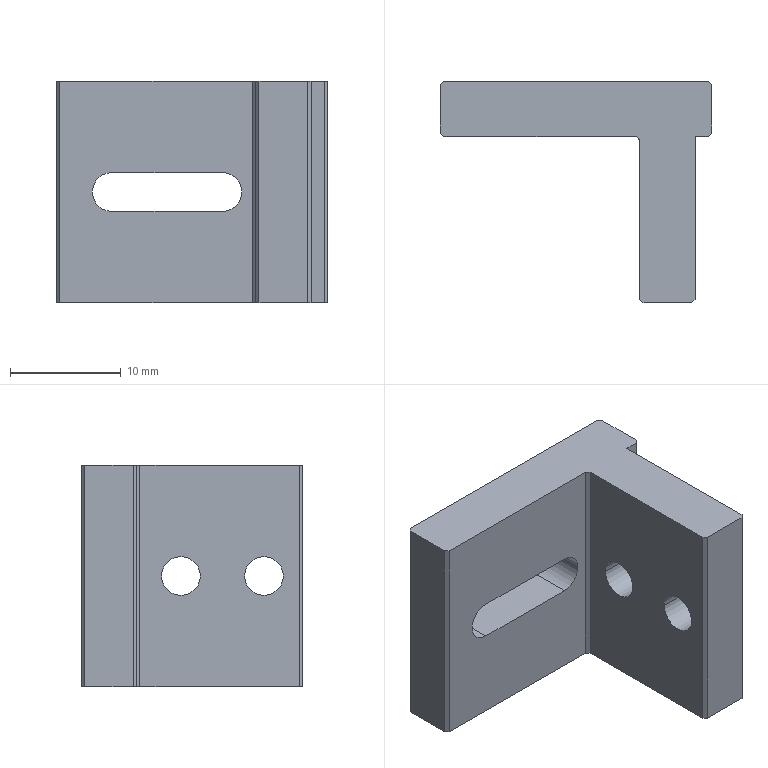Part | SolidWorks | features ICE 2, Extrusion 1 | 1 solid | 26 faces | box 24.5 x 20 x 20 mm | volume 3626 mm3 | plane 19 | cylinder 7 | commonest cylinder face diameters 3.5 x7
STEP:
#1=CARTESIAN_POINT('',(-9.5,5.,11.75));
#2=VERTEX_POINT('',#1);
#3=CARTESIAN_POINT('',(-7.75,5.,10.));
#4=VERTEX_POINT('',#3);
#5=CARTESIAN_POINT('',(-9.5,5.,10.));
#6=DIRECTION('',(0.,1.,0.));
#7=DIRECTION('',(1.,0.,0.));
#8=AXIS2_PLACEMENT_3D('',#5,#6,#7);
#9=CIRCLE('',#8,1.75);
#10=EDGE_CURVE('',#2,#4,#9,.T.);
#11=ORIENTED_EDGE('',*,*,#10,.T.);
#12=CARTESIAN_POINT('',(-7.75,0.,10.));
#13=VERTEX_POINT('',#12);
#14=CARTESIAN_POINT('',(-7.75,5.001,10.));
#15=DIRECTION('',(0.,-1.,0.));
#16=VECTOR('',#15,1000.);
#17=LINE('',#14,#16);
#18=EDGE_CURVE('',#4,#13,#17,.T.);
#19=ORIENTED_EDGE('',*,*,#18,.T.);
#20=CARTESIAN_POINT('',(-9.5,0.,11.75));
#21=VERTEX_POINT('',#20);
#22=CARTESIAN_POINT('',(-9.5,0.,10.));
#23=DIRECTION('',(0.,-1.,0.));
#24=DIRECTION('',(1.,0.,0.));
#25=AXIS2_PLACEMENT_3D('',#22,#23,#24);
#26=CIRCLE('',#25,1.75);
#27=EDGE_CURVE('',#13,#21,#26,.T.);
#28=ORIENTED_EDGE('',*,*,#27,.T.);
#29=CARTESIAN_POINT('',(-9.5,5.001,11.75));
#30=DIRECTION('',(0.,-1.,0.));
#31=VECTOR('',#30,1000.);
#32=LINE('',#29,#31);
#33=EDGE_CURVE('',#2,#21,#32,.T.);
#34=ORIENTED_EDGE('',*,*,#33,.F.);
#35=EDGE_LOOP('',(#11,#19,#28,#34));
#36=FACE_OUTER_BOUND('',#35,.T.);
#37=CARTESIAN_POINT('',(-9.5,5.001,10.));
#38=DIRECTION('',(0.,-1.,0.));
#39=DIRECTION('',(1.,0.,0.));
#40=AXIS2_PLACEMENT_3D('',#37,#38,#39);
#41=CYLINDRICAL_SURFACE('',#40,1.75);
#42=ADVANCED_FACE('',(#36),#41,.F.);
#43=CARTESIAN_POINT('',(-6.5,-9.75,10.));
#44=VERTEX_POINT('',#43);
#45=CARTESIAN_POINT('',(-6.5,-13.25,10.));
#46=VERTEX_POINT('',#45);
#47=CARTESIAN_POINT('',(-6.5,-11.5,10.));
#48=DIRECTION('',(-1.,0.,0.));
#49=DIRECTION('',(0.,1.,0.));
#50=AXIS2_PLACEMENT_3D('',#47,#48,#49);
#51=CIRCLE('',#50,1.75);
#52=EDGE_CURVE('',#44,#46,#51,.T.);
#53=ORIENTED_EDGE('',*,*,#52,.T.);
#54=CARTESIAN_POINT('',(-1.5,-13.25,10.));
#55=VERTEX_POINT('',#54);
#56=CARTESIAN_POINT('',(-24.501,-13.25,10.));
#57=DIRECTION('',(1.,0.,0.));
#58=VECTOR('',#57,1000.);
#59=LINE('',#56,#58);
#60=EDGE_CURVE('',#46,#55,#59,.T.);
#61=ORIENTED_EDGE('',*,*,#60,.T.);
#62=CARTESIAN_POINT('',(-1.5,-9.75,10.));
#63=VERTEX_POINT('',#62);
#64=CARTESIAN_POINT('',(-1.5,-11.5,10.));
#65=DIRECTION('',(1.,0.,0.));
#66=DIRECTION('',(0.,1.,0.));
#67=AXIS2_PLACEMENT_3D('',#64,#65,#66);
#68=CIRCLE('',#67,1.75);
#69=EDGE_CURVE('',#55,#63,#68,.T.);
#70=ORIENTED_EDGE('',*,*,#69,.T.);
#71=CARTESIAN_POINT('',(-24.501,-9.75,10.));
#72=DIRECTION('',(1.,0.,0.));
#73=VECTOR('',#72,1000.);
#74=LINE('',#71,#73);
#75=EDGE_CURVE('',#44,#63,#74,.T.);
#76=ORIENTED_EDGE('',*,*,#75,.F.);
#77=EDGE_LOOP('',(#53,#61,#70,#76));
#78=FACE_OUTER_BOUND('',#77,.T.);
#79=CARTESIAN_POINT('',(-24.501,-11.5,10.));
#80=DIRECTION('',(1.,0.,0.));
#81=DIRECTION('',(0.,1.,0.));
#82=AXIS2_PLACEMENT_3D('',#79,#80,#81);
#83=CYLINDRICAL_SURFACE('',#82,1.75);
#84=ADVANCED_FACE('',(#78),#83,.F.);
#85=CARTESIAN_POINT('',(-6.5,-2.25,10.));
#86=VERTEX_POINT('',#85);
#87=CARTESIAN_POINT('',(-6.5,-5.75,10.));
#88=VERTEX_POINT('',#87);
#89=CARTESIAN_POINT('',(-6.5,-4.,10.));
#90=DIRECTION('',(-1.,0.,0.));
#91=DIRECTION('',(0.,1.,0.));
#92=AXIS2_PLACEMENT_3D('',#89,#90,#91);
#93=CIRCLE('',#92,1.75);
#94=EDGE_CURVE('',#86,#88,#93,.T.);
#95=ORIENTED_EDGE('',*,*,#94,.T.);
#96=CARTESIAN_POINT('',(-1.5,-5.75,10.));
#97=VERTEX_POINT('',#96);
#98=CARTESIAN_POINT('',(-24.501,-5.75,10.));
#99=DIRECTION('',(1.,0.,0.));
#100=VECTOR('',#99,1000.);
#101=LINE('',#98,#100);
#102=EDGE_CURVE('',#88,#97,#101,.T.);
#103=ORIENTED_EDGE('',*,*,#102,.T.);
#104=CARTESIAN_POINT('',(-1.5,-2.25,10.));
#105=VERTEX_POINT('',#104);
#106=CARTESIAN_POINT('',(-1.5,-4.,10.));
#107=DIRECTION('',(1.,0.,0.));
#108=DIRECTION('',(0.,-1.,0.));
#109=AXIS2_PLACEMENT_3D('',#106,#107,#108);
#110=CIRCLE('',#109,1.75);
#111=EDGE_CURVE('',#97,#105,#110,.T.);
#112=ORIENTED_EDGE('',*,*,#111,.T.);
#113=CARTESIAN_POINT('',(-24.501,-2.25,10.));
#114=DIRECTION('',(1.,0.,0.));
#115=VECTOR('',#114,1000.);
#116=LINE('',#113,#115);
#117=EDGE_CURVE('',#86,#105,#116,.T.);
#118=ORIENTED_EDGE('',*,*,#117,.F.);
#119=EDGE_LOOP('',(#95,#103,#112,#118));
#120=FACE_OUTER_BOUND('',#119,.T.);
#121=CARTESIAN_POINT('',(-24.501,-4.,10.));
#122=DIRECTION('',(1.,0.,0.));
#123=DIRECTION('',(0.,1.,0.));
#124=AXIS2_PLACEMENT_3D('',#121,#122,#123);
#125=CYLINDRICAL_SURFACE('',#124,1.75);
#126=ADVANCED_FACE('',(#120),#125,.F.);
#127=CARTESIAN_POINT('',(-1.5,-11.5,10.));
#128=DIRECTION('',(1.,0.,0.));
#129=DIRECTION('',(0.,1.,0.));
#130=AXIS2_PLACEMENT_3D('',#127,#128,#129);
#131=CIRCLE('',#130,1.75);
#132=EDGE_CURVE('',#63,#55,#131,.T.);
#133=ORIENTED_EDGE('',*,*,#132,.F.);
#134=ORIENTED_EDGE('',*,*,#69,.F.);
#135=EDGE_LOOP('',(#133,#134));
#136=FACE_BOUND('',#135,.T.);
#137=CARTESIAN_POINT('',(-1.5,-4.,10.));
#138=DIRECTION('',(1.,0.,0.));
#139=DIRECTION('',(0.,-1.,0.));
#140=AXIS2_PLACEMENT_3D('',#137,#138,#139);
#141=CIRCLE('',#140,1.75);
#142=EDGE_CURVE('',#105,#97,#141,.T.);
#143=ORIENTED_EDGE('',*,*,#142,.F.);
#144=ORIENTED_EDGE('',*,*,#111,.F.);
#145=EDGE_LOOP('',(#143,#144));
#146=FACE_BOUND('',#145,.T.);
#147=CARTESIAN_POINT('',(-1.5,-14.7,0.));
#148=VERTEX_POINT('',#147);
#149=CARTESIAN_POINT('',(-1.5,0.,0.));
#150=VERTEX_POINT('',#149);
#151=CARTESIAN_POINT('',(-1.5,0.,0.));
#152=DIRECTION('',(0.,1.,0.));
#153=VECTOR('',#152,1000.);
#154=LINE('',#151,#153);
#155=EDGE_CURVE('',#148,#150,#154,.T.);
#156=ORIENTED_EDGE('',*,*,#155,.T.);
#157=CARTESIAN_POINT('',(-1.5,0.,20.));
#158=VERTEX_POINT('',#157);
#159=CARTESIAN_POINT('',(-1.5,0.,20.));
#160=DIRECTION('',(0.,0.,-1.));
#161=VECTOR('',#160,1000.);
#162=LINE('',#159,#161);
#163=EDGE_CURVE('',#158,#150,#162,.T.);
#164=ORIENTED_EDGE('',*,*,#163,.F.);
#165=CARTESIAN_POINT('',(-1.5,-14.7,20.));
#166=VERTEX_POINT('',#165);
#167=CARTESIAN_POINT('',(-1.5,0.,20.));
#168=DIRECTION('',(0.,1.,0.));
#169=VECTOR('',#168,1000.);
#170=LINE('',#167,#169);
#171=EDGE_CURVE('',#166,#158,#170,.T.);
#172=ORIENTED_EDGE('',*,*,#171,.F.);
#173=CARTESIAN_POINT('',(-1.5,-14.7,20.));
#174=DIRECTION('',(0.,0.,-1.));
#175=VECTOR('',#174,1000.);
#176=LINE('',#173,#175);
#177=EDGE_CURVE('',#166,#148,#176,.T.);
#178=ORIENTED_EDGE('',*,*,#177,.T.);
#179=EDGE_LOOP('',(#156,#164,#172,#178));
#180=FACE_OUTER_BOUND('',#179,.T.);
#181=CARTESIAN_POINT('',(-1.5,0.,20.));
#182=DIRECTION('',(-1.,0.,0.));
#183=DIRECTION('',(0.,-1.,0.));
#184=AXIS2_PLACEMENT_3D('',#181,#182,#183);
#185=PLANE('',#184);
#186=ADVANCED_FACE('',(#136,#146,#180),#185,.F.);
#187=CARTESIAN_POINT('',(-0.3,0.,0.));
#188=VERTEX_POINT('',#187);
#189=CARTESIAN_POINT('',(-0.3,0.,0.));
#190=DIRECTION('',(1.,0.,0.));
#191=VECTOR('',#190,1000.);
#192=LINE('',#189,#191);
#193=EDGE_CURVE('',#150,#188,#192,.T.);
#194=ORIENTED_EDGE('',*,*,#193,.T.);
#195=CARTESIAN_POINT('',(-0.3,0.,20.));
#196=VERTEX_POINT('',#195);
#197=CARTESIAN_POINT('',(-0.3,0.,20.));
#198=DIRECTION('',(0.,0.,-1.));
#199=VECTOR('',#198,1000.);
#200=LINE('',#197,#199);
#201=EDGE_CURVE('',#196,#188,#200,.T.);
#202=ORIENTED_EDGE('',*,*,#201,.F.);
#203=CARTESIAN_POINT('',(-0.3,0.,20.));
#204=DIRECTION('',(1.,0.,0.));
#205=VECTOR('',#204,1000.);
#206=LINE('',#203,#205);
#207=EDGE_CURVE('',#158,#196,#206,.T.);
#208=ORIENTED_EDGE('',*,*,#207,.F.);
#209=ORIENTED_EDGE('',*,*,#163,.T.);
#210=EDGE_LOOP('',(#194,#202,#208,#209));
#211=FACE_OUTER_BOUND('',#210,.T.);
#212=CARTESIAN_POINT('',(-0.3,0.,20.));
#213=DIRECTION('',(0.,1.,0.));
#214=DIRECTION('',(-1.,0.,0.));
#215=AXIS2_PLACEMENT_3D('',#212,#213,#214);
#216=PLANE('',#215);
#217=ADVANCED_FACE('',(#211),#216,.F.);
#218=CARTESIAN_POINT('',(0.,0.3,0.));
#219=VERTEX_POINT('',#218);
#220=CARTESIAN_POINT('',(0.,0.3,0.));
#221=DIRECTION('',(0.7071,0.7071,0.));
#222=VECTOR('',#221,1000.);
#223=LINE('',#220,#222);
#224=EDGE_CURVE('',#188,#219,#223,.T.);
#225=ORIENTED_EDGE('',*,*,#224,.T.);
#226=CARTESIAN_POINT('',(0.,0.3,20.));
#227=VERTEX_POINT('',#226);
#228=CARTESIAN_POINT('',(0.,0.3,20.));
#229=DIRECTION('',(0.,0.,-1.));
#230=VECTOR('',#229,1000.);
#231=LINE('',#228,#230);
#232=EDGE_CURVE('',#227,#219,#231,.T.);
#233=ORIENTED_EDGE('',*,*,#232,.F.);
#234=CARTESIAN_POINT('',(0.,0.3,20.));
#235=DIRECTION('',(0.7071,0.7071,0.));
#236=VECTOR('',#235,1000.);
#237=LINE('',#234,#236);
#238=EDGE_CURVE('',#196,#227,#237,.T.);
#239=ORIENTED_EDGE('',*,*,#238,.F.);
#240=ORIENTED_EDGE('',*,*,#201,.T.);
#241=EDGE_LOOP('',(#225,#233,#239,#240));
#242=FACE_OUTER_BOUND('',#241,.T.);
#243=CARTESIAN_POINT('',(0.,0.3,20.));
#244=DIRECTION('',(-0.7071,0.7071,0.));
#245=DIRECTION('',(-0.7071,-0.7071,0.));
#246=AXIS2_PLACEMENT_3D('',#243,#244,#245);
#247=PLANE('',#246);
#248=ADVANCED_FACE('',(#242),#247,.F.);
#249=CARTESIAN_POINT('',(0.,4.7,0.));
#250=VERTEX_POINT('',#249);
#251=CARTESIAN_POINT('',(0.,0.3,0.));
#252=DIRECTION('',(0.,1.,0.));
#253=VECTOR('',#252,1000.);
#254=LINE('',#251,#253);
#255=EDGE_CURVE('',#219,#250,#254,.T.);
#256=ORIENTED_EDGE('',*,*,#255,.T.);
#257=CARTESIAN_POINT('',(0.,4.7,20.));
#258=VERTEX_POINT('',#257);
#259=CARTESIAN_POINT('',(0.,4.7,20.));
#260=DIRECTION('',(0.,0.,-1.));
#261=VECTOR('',#260,1000.);
#262=LINE('',#259,#261);
#263=EDGE_CURVE('',#258,#250,#262,.T.);
#264=ORIENTED_EDGE('',*,*,#263,.F.);
#265=CARTESIAN_POINT('',(0.,0.3,20.));
#266=DIRECTION('',(0.,1.,0.));
#267=VECTOR('',#266,1000.);
#268=LINE('',#265,#267);
#269=EDGE_CURVE('',#227,#258,#268,.T.);
#270=ORIENTED_EDGE('',*,*,#269,.F.);
#271=ORIENTED_EDGE('',*,*,#232,.T.);
#272=EDGE_LOOP('',(#256,#264,#270,#271));
#273=FACE_OUTER_BOUND('',#272,.T.);
#274=CARTESIAN_POINT('',(0.,0.3,20.));
#275=DIRECTION('',(-1.,0.,0.));
#276=DIRECTION('',(0.,0.,1.));
#277=AXIS2_PLACEMENT_3D('',#274,#275,#276);
#278=PLANE('',#277);
#279=ADVANCED_FACE('',(#273),#278,.F.);
#280=CARTESIAN_POINT('',(-0.3,5.,0.));
#281=VERTEX_POINT('',#280);
#282=CARTESIAN_POINT('',(0.,4.7,0.));
#283=DIRECTION('',(-0.7071,0.7071,0.));
#284=VECTOR('',#283,1000.);
#285=LINE('',#282,#284);
#286=EDGE_CURVE('',#250,#281,#285,.T.);
#287=ORIENTED_EDGE('',*,*,#286,.T.);
#288=CARTESIAN_POINT('',(-0.3,5.,20.));
#289=VERTEX_POINT('',#288);
#290=CARTESIAN_POINT('',(-0.3,5.,20.));
#291=DIRECTION('',(0.,0.,-1.));
#292=VECTOR('',#291,1000.);
#293=LINE('',#290,#292);
#294=EDGE_CURVE('',#289,#281,#293,.T.);
#295=ORIENTED_EDGE('',*,*,#294,.F.);
#296=CARTESIAN_POINT('',(0.,4.7,20.));
#297=DIRECTION('',(-0.7071,0.7071,0.));
#298=VECTOR('',#297,1000.);
#299=LINE('',#296,#298);
#300=EDGE_CURVE('',#258,#289,#299,.T.);
#301=ORIENTED_EDGE('',*,*,#300,.F.);
#302=ORIENTED_EDGE('',*,*,#263,.T.);
#303=EDGE_LOOP('',(#287,#295,#301,#302));
#304=FACE_OUTER_BOUND('',#303,.T.);
#305=CARTESIAN_POINT('',(0.,4.7,20.));
#306=DIRECTION('',(-0.7071,-0.7071,0.));
#307=DIRECTION('',(0.7071,-0.7071,0.));
#308=AXIS2_PLACEMENT_3D('',#305,#306,#307);
#309=PLANE('',#308);
#310=ADVANCED_FACE('',(#304),#309,.F.);
#311=CARTESIAN_POINT('',(-19.5,5.,11.75));
#312=VERTEX_POINT('',#311);
#313=CARTESIAN_POINT('',(-19.5,5.,11.75));
#314=DIRECTION('',(1.,0.,0.));
#315=VECTOR('',#314,1000.);
#316=LINE('',#313,#315);
#317=EDGE_CURVE('',#312,#2,#316,.T.);
#318=ORIENTED_EDGE('',*,*,#317,.F.);
#319=CARTESIAN_POINT('',(-19.5,5.,8.25));
#320=VERTEX_POINT('',#319);
#321=CARTESIAN_POINT('',(-19.5,5.,10.));
#322=DIRECTION('',(0.,1.,0.));
#323=DIRECTION('',(1.,0.,0.));
#324=AXIS2_PLACEMENT_3D('',#321,#322,#323);
#325=CIRCLE('',#324,1.75);
#326=EDGE_CURVE('',#320,#312,#325,.T.);
#327=ORIENTED_EDGE('',*,*,#326,.F.);
#328=CARTESIAN_POINT('',(-9.5,5.,8.25));
#329=VERTEX_POINT('',#328);
#330=CARTESIAN_POINT('',(-19.5,5.,8.25));
#331=DIRECTION('',(-1.,0.,0.));
#332=VECTOR('',#331,1000.);
#333=LINE('',#330,#332);
#334=EDGE_CURVE('',#329,#320,#333,.T.);
#335=ORIENTED_EDGE('',*,*,#334,.F.);
#336=CARTESIAN_POINT('',(-9.5,5.,10.));
#337=DIRECTION('',(0.,1.,0.));
#338=DIRECTION('',(1.,0.,0.));
#339=AXIS2_PLACEMENT_3D('',#336,#337,#338);
#340=CIRCLE('',#339,1.75);
#341=EDGE_CURVE('',#4,#329,#340,.T.);
#342=ORIENTED_EDGE('',*,*,#341,.F.);
#343=ORIENTED_EDGE('',*,*,#10,.F.);
#344=EDGE_LOOP('',(#318,#327,#335,#342,#343));
#345=FACE_BOUND('',#344,.T.);
#346=CARTESIAN_POINT('',(-24.2,5.,0.));
#347=VERTEX_POINT('',#346);
#348=CARTESIAN_POINT('',(-0.3,5.,0.));
#349=DIRECTION('',(-1.,0.,0.));
#350=VECTOR('',#349,1000.);
#351=LINE('',#348,#350);
#352=EDGE_CURVE('',#281,#347,#351,.T.);
#353=ORIENTED_EDGE('',*,*,#352,.T.);
#354=CARTESIAN_POINT('',(-24.2,5.,20.));
#355=VERTEX_POINT('',#354);
#356=CARTESIAN_POINT('',(-24.2,5.,20.));
#357=DIRECTION('',(0.,0.,-1.));
#358=VECTOR('',#357,1000.);
#359=LINE('',#356,#358);
#360=EDGE_CURVE('',#355,#347,#359,.T.);
#361=ORIENTED_EDGE('',*,*,#360,.F.);
#362=CARTESIAN_POINT('',(-0.3,5.,20.));
#363=DIRECTION('',(-1.,0.,0.));
#364=VECTOR('',#363,1000.);
#365=LINE('',#362,#364);
#366=EDGE_CURVE('',#289,#355,#365,.T.);
#367=ORIENTED_EDGE('',*,*,#366,.F.);
#368=ORIENTED_EDGE('',*,*,#294,.T.);
#369=EDGE_LOOP('',(#353,#361,#367,#368));
#370=FACE_OUTER_BOUND('',#369,.T.);
#371=CARTESIAN_POINT('',(-0.3,5.,20.));
#372=DIRECTION('',(0.,-1.,0.));
#373=DIRECTION('',(1.,0.,0.));
#374=AXIS2_PLACEMENT_3D('',#371,#372,#373);
#375=PLANE('',#374);
#376=ADVANCED_FACE('',(#345,#370),#375,.F.);
#377=CARTESIAN_POINT('',(-24.5,4.7,0.));
#378=VERTEX_POINT('',#377);
#379=CARTESIAN_POINT('',(-24.2,5.,0.));
#380=DIRECTION('',(-0.7071,-0.7071,0.));
#381=VECTOR('',#380,1000.);
#382=LINE('',#379,#381);
#383=EDGE_CURVE('',#347,#378,#382,.T.);
#384=ORIENTED_EDGE('',*,*,#383,.T.);
#385=CARTESIAN_POINT('',(-24.5,4.7,20.));
#386=VERTEX_POINT('',#385);
#387=CARTESIAN_POINT('',(-24.5,4.7,20.));
#388=DIRECTION('',(0.,0.,-1.));
#389=VECTOR('',#388,1000.);
#390=LINE('',#387,#389);
#391=EDGE_CURVE('',#386,#378,#390,.T.);
#392=ORIENTED_EDGE('',*,*,#391,.F.);
#393=CARTESIAN_POINT('',(-24.2,5.,20.));
#394=DIRECTION('',(-0.7071,-0.7071,0.));
#395=VECTOR('',#394,1000.);
#396=LINE('',#393,#395);
#397=EDGE_CURVE('',#355,#386,#396,.T.);
#398=ORIENTED_EDGE('',*,*,#397,.F.);
#399=ORIENTED_EDGE('',*,*,#360,.T.);
#400=EDGE_LOOP('',(#384,#392,#398,#399));
#401=FACE_OUTER_BOUND('',#400,.T.);
#402=CARTESIAN_POINT('',(-24.2,5.,20.));
#403=DIRECTION('',(0.7071,-0.7071,0.));
#404=DIRECTION('',(0.7071,0.7071,0.));
#405=AXIS2_PLACEMENT_3D('',#402,#403,#404);
#406=PLANE('',#405);
#407=ADVANCED_FACE('',(#401),#406,.F.);
#408=CARTESIAN_POINT('',(-24.5,0.3,0.));
#409=VERTEX_POINT('',#408);
#410=CARTESIAN_POINT('',(-24.5,0.3,0.));
#411=DIRECTION('',(0.,-1.,0.));
#412=VECTOR('',#411,1000.);
#413=LINE('',#410,#412);
#414=EDGE_CURVE('',#378,#409,#413,.T.);
#415=ORIENTED_EDGE('',*,*,#414,.T.);
#416=CARTESIAN_POINT('',(-24.5,0.3,20.));
#417=VERTEX_POINT('',#416);
#418=CARTESIAN_POINT('',(-24.5,0.3,20.));
#419=DIRECTION('',(0.,0.,-1.));
#420=VECTOR('',#419,1000.);
#421=LINE('',#418,#420);
#422=EDGE_CURVE('',#417,#409,#421,.T.);
#423=ORIENTED_EDGE('',*,*,#422,.F.);
#424=CARTESIAN_POINT('',(-24.5,0.3,20.));
#425=DIRECTION('',(0.,-1.,0.));
#426=VECTOR('',#425,1000.);
#427=LINE('',#424,#426);
#428=EDGE_CURVE('',#386,#417,#427,.T.);
#429=ORIENTED_EDGE('',*,*,#428,.F.);
#430=ORIENTED_EDGE('',*,*,#391,.T.);
#431=EDGE_LOOP('',(#415,#423,#429,#430));
#432=FACE_OUTER_BOUND('',#431,.T.);
#433=CARTESIAN_POINT('',(-24.5,0.3,20.));
#434=DIRECTION('',(1.,0.,0.));
#435=DIRECTION('',(0.,0.,-1.));
#436=AXIS2_PLACEMENT_3D('',#433,#434,#435);
#437=PLANE('',#436);
#438=ADVANCED_FACE('',(#432),#437,.F.);
#439=CARTESIAN_POINT('',(-24.2,0.,0.));
#440=VERTEX_POINT('',#439);
#441=CARTESIAN_POINT('',(-24.2,0.,0.));
#442=DIRECTION('',(0.7071,-0.7071,0.));
#443=VECTOR('',#442,1000.);
#444=LINE('',#441,#443);
#445=EDGE_CURVE('',#409,#440,#444,.T.);
#446=ORIENTED_EDGE('',*,*,#445,.T.);
#447=CARTESIAN_POINT('',(-24.2,0.,20.));
#448=VERTEX_POINT('',#447);
#449=CARTESIAN_POINT('',(-24.2,0.,20.));
#450=DIRECTION('',(0.,0.,-1.));
#451=VECTOR('',#450,1000.);
#452=LINE('',#449,#451);
#453=EDGE_CURVE('',#448,#440,#452,.T.);
#454=ORIENTED_EDGE('',*,*,#453,.F.);
#455=CARTESIAN_POINT('',(-24.2,0.,20.));
#456=DIRECTION('',(0.7071,-0.7071,0.));
#457=VECTOR('',#456,1000.);
#458=LINE('',#455,#457);
#459=EDGE_CURVE('',#417,#448,#458,.T.);
#460=ORIENTED_EDGE('',*,*,#459,.F.);
#461=ORIENTED_EDGE('',*,*,#422,.T.);
#462=EDGE_LOOP('',(#446,#454,#460,#461));
#463=FACE_OUTER_BOUND('',#462,.T.);
#464=CARTESIAN_POINT('',(-24.2,0.,20.));
#465=DIRECTION('',(0.7071,0.7071,0.));
#466=DIRECTION('',(-0.7071,0.7071,0.));
#467=AXIS2_PLACEMENT_3D('',#464,#465,#466);
#468=PLANE('',#467);
#469=ADVANCED_FACE('',(#463),#468,.F.);
#470=CARTESIAN_POINT('',(-19.5,0.,8.25));
#471=VERTEX_POINT('',#470);
#472=CARTESIAN_POINT('',(-9.5,0.,8.25));
#473=VERTEX_POINT('',#472);
#474=CARTESIAN_POINT('',(-19.5,0.,8.25));
#475=DIRECTION('',(1.,0.,0.));
#476=VECTOR('',#475,1000.);
#477=LINE('',#474,#476);
#478=EDGE_CURVE('',#471,#473,#477,.T.);
#479=ORIENTED_EDGE('',*,*,#478,.F.);
#480=CARTESIAN_POINT('',(-19.5,0.,11.75));
#481=VERTEX_POINT('',#480);
#482=CARTESIAN_POINT('',(-19.5,0.,10.));
#483=DIRECTION('',(0.,-1.,0.));
#484=DIRECTION('',(1.,0.,0.));
#485=AXIS2_PLACEMENT_3D('',#482,#483,#484);
#486=CIRCLE('',#485,1.75);
#487=EDGE_CURVE('',#481,#471,#486,.T.);
#488=ORIENTED_EDGE('',*,*,#487,.F.);
#489=CARTESIAN_POINT('',(-19.5,0.,11.75));
#490=DIRECTION('',(-1.,0.,0.));
#491=VECTOR('',#490,1000.);
#492=LINE('',#489,#491);
#493=EDGE_CURVE('',#21,#481,#492,.T.);
#494=ORIENTED_EDGE('',*,*,#493,.F.);
#495=ORIENTED_EDGE('',*,*,#27,.F.);
#496=CARTESIAN_POINT('',(-9.5,0.,10.));
#497=DIRECTION('',(0.,-1.,0.));
#498=DIRECTION('',(1.,0.,0.));
#499=AXIS2_PLACEMENT_3D('',#496,#497,#498);
#500=CIRCLE('',#499,1.75);
#501=EDGE_CURVE('',#473,#13,#500,.T.);
#502=ORIENTED_EDGE('',*,*,#501,.F.);
#503=EDGE_LOOP('',(#479,#488,#494,#495,#502));
#504=FACE_BOUND('',#503,.T.);
#505=CARTESIAN_POINT('',(-6.8,0.,0.));
#506=VERTEX_POINT('',#505);
#507=CARTESIAN_POINT('',(-6.8,0.,0.));
#508=DIRECTION('',(1.,0.,0.));
#509=VECTOR('',#508,1000.);
#510=LINE('',#507,#509);
#511=EDGE_CURVE('',#440,#506,#510,.T.);
#512=ORIENTED_EDGE('',*,*,#511,.T.);
#513=CARTESIAN_POINT('',(-6.8,0.,20.));
#514=VERTEX_POINT('',#513);
#515=CARTESIAN_POINT('',(-6.8,0.,20.));
#516=DIRECTION('',(0.,0.,-1.));
#517=VECTOR('',#516,1000.);
#518=LINE('',#515,#517);
#519=EDGE_CURVE('',#514,#506,#518,.T.);
#520=ORIENTED_EDGE('',*,*,#519,.F.);
#521=CARTESIAN_POINT('',(-6.8,0.,20.));
#522=DIRECTION('',(1.,0.,0.));
#523=VECTOR('',#522,1000.);
#524=LINE('',#521,#523);
#525=EDGE_CURVE('',#448,#514,#524,.T.);
#526=ORIENTED_EDGE('',*,*,#525,.F.);
#527=ORIENTED_EDGE('',*,*,#453,.T.);
#528=EDGE_LOOP('',(#512,#520,#526,#527));
#529=FACE_OUTER_BOUND('',#528,.T.);
#530=CARTESIAN_POINT('',(-6.8,0.,20.));
#531=DIRECTION('',(0.,1.,0.));
#532=DIRECTION('',(-1.,0.,0.));
#533=AXIS2_PLACEMENT_3D('',#530,#531,#532);
#534=PLANE('',#533);
#535=ADVANCED_FACE('',(#504,#529),#534,.F.);
#536=CARTESIAN_POINT('',(-6.5,-0.3,0.));
#537=VERTEX_POINT('',#536);
#538=CARTESIAN_POINT('',(-6.5,-0.3,0.));
#539=DIRECTION('',(0.7071,-0.7071,0.));
#540=VECTOR('',#539,1000.);
#541=LINE('',#538,#540);
#542=EDGE_CURVE('',#506,#537,#541,.T.);
#543=ORIENTED_EDGE('',*,*,#542,.T.);
#544=CARTESIAN_POINT('',(-6.5,-0.3,20.));
#545=VERTEX_POINT('',#544);
#546=CARTESIAN_POINT('',(-6.5,-0.3,20.));
#547=DIRECTION('',(0.,0.,-1.));
#548=VECTOR('',#547,1000.);
#549=LINE('',#546,#548);
#550=EDGE_CURVE('',#545,#537,#549,.T.);
#551=ORIENTED_EDGE('',*,*,#550,.F.);
#552=CARTESIAN_POINT('',(-6.5,-0.3,20.));
#553=DIRECTION('',(0.7071,-0.7071,0.));
#554=VECTOR('',#553,1000.);
#555=LINE('',#552,#554);
#556=EDGE_CURVE('',#514,#545,#555,.T.);
#557=ORIENTED_EDGE('',*,*,#556,.F.);
#558=ORIENTED_EDGE('',*,*,#519,.T.);
#559=EDGE_LOOP('',(#543,#551,#557,#558));
#560=FACE_OUTER_BOUND('',#559,.T.);
#561=CARTESIAN_POINT('',(-6.5,-0.3,20.));
#562=DIRECTION('',(0.7071,0.7071,0.));
#563=DIRECTION('',(-0.7071,0.7071,0.));
#564=AXIS2_PLACEMENT_3D('',#561,#562,#563);
#565=PLANE('',#564);
#566=ADVANCED_FACE('',(#560),#565,.F.);
#567=ORIENTED_EDGE('',*,*,#52,.F.);
#568=CARTESIAN_POINT('',(-6.5,-11.5,10.));
#569=DIRECTION('',(-1.,0.,0.));
#570=DIRECTION('',(0.,1.,0.));
#571=AXIS2_PLACEMENT_3D('',#568,#569,#570);
#572=CIRCLE('',#571,1.75);
#573=EDGE_CURVE('',#46,#44,#572,.T.);
#574=ORIENTED_EDGE('',*,*,#573,.F.);
#575=EDGE_LOOP('',(#567,#574));
#576=FACE_BOUND('',#575,.T.);
#577=ORIENTED_EDGE('',*,*,#94,.F.);
#578=CARTESIAN_POINT('',(-6.5,-4.,10.));
#579=DIRECTION('',(-1.,0.,0.));
#580=DIRECTION('',(0.,1.,0.));
#581=AXIS2_PLACEMENT_3D('',#578,#579,#580);
#582=CIRCLE('',#581,1.75);
#583=EDGE_CURVE('',#88,#86,#582,.T.);
#584=ORIENTED_EDGE('',*,*,#583,.F.);
#585=EDGE_LOOP('',(#577,#584));
#586=FACE_BOUND('',#585,.T.);
#587=CARTESIAN_POINT('',(-6.5,-14.7,0.));
#588=VERTEX_POINT('',#587);
#589=CARTESIAN_POINT('',(-6.5,-0.3,0.));
#590=DIRECTION('',(0.,-1.,0.));
#591=VECTOR('',#590,1000.);
#592=LINE('',#589,#591);
#593=EDGE_CURVE('',#537,#588,#592,.T.);
#594=ORIENTED_EDGE('',*,*,#593,.T.);
#595=CARTESIAN_POINT('',(-6.5,-14.7,20.));
#596=VERTEX_POINT('',#595);
#597=CARTESIAN_POINT('',(-6.5,-14.7,20.));
#598=DIRECTION('',(0.,0.,-1.));
#599=VECTOR('',#598,1000.);
#600=LINE('',#597,#599);
#601=EDGE_CURVE('',#596,#588,#600,.T.);
#602=ORIENTED_EDGE('',*,*,#601,.F.);
#603=CARTESIAN_POINT('',(-6.5,-0.3,20.));
#604=DIRECTION('',(0.,-1.,0.));
#605=VECTOR('',#604,1000.);
#606=LINE('',#603,#605);
#607=EDGE_CURVE('',#545,#596,#606,.T.);
#608=ORIENTED_EDGE('',*,*,#607,.F.);
#609=ORIENTED_EDGE('',*,*,#550,.T.);
#610=EDGE_LOOP('',(#594,#602,#608,#609));
#611=FACE_OUTER_BOUND('',#610,.T.);
#612=CARTESIAN_POINT('',(-6.5,-0.3,20.));
#613=DIRECTION('',(1.,0.,0.));
#614=DIRECTION('',(0.,1.,0.));
#615=AXIS2_PLACEMENT_3D('',#612,#613,#614);
#616=PLANE('',#615);
#617=ADVANCED_FACE('',(#576,#586,#611),#616,.F.);
#618=CARTESIAN_POINT('',(-6.2,-15.,0.));
#619=VERTEX_POINT('',#618);
#620=CARTESIAN_POINT('',(-6.5,-14.7,0.));
#621=DIRECTION('',(0.7071,-0.7071,0.));
#622=VECTOR('',#621,1000.);
#623=LINE('',#620,#622);
#624=EDGE_CURVE('',#588,#619,#623,.T.);
#625=ORIENTED_EDGE('',*,*,#624,.T.);
#626=CARTESIAN_POINT('',(-6.2,-15.,20.));
#627=VERTEX_POINT('',#626);
#628=CARTESIAN_POINT('',(-6.2,-15.,20.));
#629=DIRECTION('',(0.,0.,-1.));
#630=VECTOR('',#629,1000.);
#631=LINE('',#628,#630);
#632=EDGE_CURVE('',#627,#619,#631,.T.);
#633=ORIENTED_EDGE('',*,*,#632,.F.);
#634=CARTESIAN_POINT('',(-6.5,-14.7,20.));
#635=DIRECTION('',(0.7071,-0.7071,0.));
#636=VECTOR('',#635,1000.);
#637=LINE('',#634,#636);
#638=EDGE_CURVE('',#596,#627,#637,.T.);
#639=ORIENTED_EDGE('',*,*,#638,.F.);
#640=ORIENTED_EDGE('',*,*,#601,.T.);
#641=EDGE_LOOP('',(#625,#633,#639,#640));
#642=FACE_OUTER_BOUND('',#641,.T.);
#643=CARTESIAN_POINT('',(-6.5,-14.7,20.));
#644=DIRECTION('',(0.7071,0.7071,0.));
#645=DIRECTION('',(-0.7071,0.7071,0.));
#646=AXIS2_PLACEMENT_3D('',#643,#644,#645);
#647=PLANE('',#646);
#648=ADVANCED_FACE('',(#642),#647,.F.);
#649=CARTESIAN_POINT('',(-1.8,-15.,0.));
#650=VERTEX_POINT('',#649);
#651=CARTESIAN_POINT('',(-6.2,-15.,0.));
#652=DIRECTION('',(1.,0.,0.));
#653=VECTOR('',#652,1000.);
#654=LINE('',#651,#653);
#655=EDGE_CURVE('',#619,#650,#654,.T.);
#656=ORIENTED_EDGE('',*,*,#655,.T.);
#657=CARTESIAN_POINT('',(-1.8,-15.,20.));
#658=VERTEX_POINT('',#657);
#659=CARTESIAN_POINT('',(-1.8,-15.,20.));
#660=DIRECTION('',(0.,0.,-1.));
#661=VECTOR('',#660,1000.);
#662=LINE('',#659,#661);
#663=EDGE_CURVE('',#658,#650,#662,.T.);
#664=ORIENTED_EDGE('',*,*,#663,.F.);
#665=CARTESIAN_POINT('',(-6.2,-15.,20.));
#666=DIRECTION('',(1.,0.,0.));
#667=VECTOR('',#666,1000.);
#668=LINE('',#665,#667);
#669=EDGE_CURVE('',#627,#658,#668,.T.);
#670=ORIENTED_EDGE('',*,*,#669,.F.);
#671=ORIENTED_EDGE('',*,*,#632,.T.);
#672=EDGE_LOOP('',(#656,#664,#670,#671));
#673=FACE_OUTER_BOUND('',#672,.T.);
#674=CARTESIAN_POINT('',(-6.2,-15.,20.));
#675=DIRECTION('',(0.,1.,0.));
#676=DIRECTION('',(0.,0.,1.));
#677=AXIS2_PLACEMENT_3D('',#674,#675,#676);
#678=PLANE('',#677);
#679=ADVANCED_FACE('',(#673),#678,.F.);
#680=CARTESIAN_POINT('',(-1.8,-15.,0.));
#681=DIRECTION('',(0.7071,0.7071,0.));
#682=VECTOR('',#681,1000.);
#683=LINE('',#680,#682);
#684=EDGE_CURVE('',#650,#148,#683,.T.);
#685=ORIENTED_EDGE('',*,*,#684,.T.);
#686=ORIENTED_EDGE('',*,*,#177,.F.);
#687=CARTESIAN_POINT('',(-1.8,-15.,20.));
#688=DIRECTION('',(0.7071,0.7071,0.));
#689=VECTOR('',#688,1000.);
#690=LINE('',#687,#689);
#691=EDGE_CURVE('',#658,#166,#690,.T.);
#692=ORIENTED_EDGE('',*,*,#691,.F.);
#693=ORIENTED_EDGE('',*,*,#663,.T.);
#694=EDGE_LOOP('',(#685,#686,#692,#693));
#695=FACE_OUTER_BOUND('',#694,.T.);
#696=CARTESIAN_POINT('',(-1.8,-15.,20.));
#697=DIRECTION('',(-0.7071,0.7071,0.));
#698=DIRECTION('',(-0.7071,-0.7071,0.));
#699=AXIS2_PLACEMENT_3D('',#696,#697,#698);
#700=PLANE('',#699);
#701=ADVANCED_FACE('',(#695),#700,.F.);
#702=ORIENTED_EDGE('',*,*,#171,.T.);
#703=ORIENTED_EDGE('',*,*,#207,.T.);
#704=ORIENTED_EDGE('',*,*,#238,.T.);
#705=ORIENTED_EDGE('',*,*,#269,.T.);
#706=ORIENTED_EDGE('',*,*,#300,.T.);
#707=ORIENTED_EDGE('',*,*,#366,.T.);
#708=ORIENTED_EDGE('',*,*,#397,.T.);
#709=ORIENTED_EDGE('',*,*,#428,.T.);
#710=ORIENTED_EDGE('',*,*,#459,.T.);
#711=ORIENTED_EDGE('',*,*,#525,.T.);
#712=ORIENTED_EDGE('',*,*,#556,.T.);
#713=ORIENTED_EDGE('',*,*,#607,.T.);
#714=ORIENTED_EDGE('',*,*,#638,.T.);
#715=ORIENTED_EDGE('',*,*,#669,.T.);
#716=ORIENTED_EDGE('',*,*,#691,.T.);
#717=EDGE_LOOP('',(#702,#703,#704,#705,#706,#707,#708,#709,#710,#711,#712,#713,#714,#715,#716));
#718=FACE_OUTER_BOUND('',#717,.T.);
#719=CARTESIAN_POINT('',(0.,0.,20.));
#720=DIRECTION('',(0.,0.,1.));
#721=DIRECTION('',(1.,0.,0.));
#722=AXIS2_PLACEMENT_3D('',#719,#720,#721);
#723=PLANE('',#722);
#724=ADVANCED_FACE('',(#718),#723,.T.);
#725=ORIENTED_EDGE('',*,*,#155,.F.);
#726=ORIENTED_EDGE('',*,*,#684,.F.);
#727=ORIENTED_EDGE('',*,*,#655,.F.);
#728=ORIENTED_EDGE('',*,*,#624,.F.);
#729=ORIENTED_EDGE('',*,*,#593,.F.);
#730=ORIENTED_EDGE('',*,*,#542,.F.);
#731=ORIENTED_EDGE('',*,*,#511,.F.);
#732=ORIENTED_EDGE('',*,*,#445,.F.);
#733=ORIENTED_EDGE('',*,*,#414,.F.);
#734=ORIENTED_EDGE('',*,*,#383,.F.);
#735=ORIENTED_EDGE('',*,*,#352,.F.);
#736=ORIENTED_EDGE('',*,*,#286,.F.);
#737=ORIENTED_EDGE('',*,*,#255,.F.);
#738=ORIENTED_EDGE('',*,*,#224,.F.);
#739=ORIENTED_EDGE('',*,*,#193,.F.);
#740=EDGE_LOOP('',(#725,#726,#727,#728,#729,#730,#731,#732,#733,#734,#735,#736,#737,#738,#739));
#741=FACE_OUTER_BOUND('',#740,.T.);
#742=CARTESIAN_POINT('',(0.,0.,0.));
#743=DIRECTION('',(0.,0.,1.));
#744=DIRECTION('',(1.,0.,0.));
#745=AXIS2_PLACEMENT_3D('',#742,#743,#744);
#746=PLANE('',#745);
#747=ADVANCED_FACE('',(#741),#746,.F.);
#748=ORIENTED_EDGE('',*,*,#102,.F.);
#749=ORIENTED_EDGE('',*,*,#583,.T.);
#750=ORIENTED_EDGE('',*,*,#117,.T.);
#751=ORIENTED_EDGE('',*,*,#142,.T.);
#752=EDGE_LOOP('',(#748,#749,#750,#751));
#753=FACE_OUTER_BOUND('',#752,.T.);
#754=CARTESIAN_POINT('',(-24.501,-4.,10.));
#755=DIRECTION('',(1.,0.,0.));
#756=DIRECTION('',(0.,1.,0.));
#757=AXIS2_PLACEMENT_3D('',#754,#755,#756);
#758=CYLINDRICAL_SURFACE('',#757,1.75);
#759=ADVANCED_FACE('',(#753),#758,.F.);
#760=ORIENTED_EDGE('',*,*,#60,.F.);
#761=ORIENTED_EDGE('',*,*,#573,.T.);
#762=ORIENTED_EDGE('',*,*,#75,.T.);
#763=ORIENTED_EDGE('',*,*,#132,.T.);
#764=EDGE_LOOP('',(#760,#761,#762,#763));
#765=FACE_OUTER_BOUND('',#764,.T.);
#766=CARTESIAN_POINT('',(-24.501,-11.5,10.));
#767=DIRECTION('',(1.,0.,0.));
#768=DIRECTION('',(0.,1.,0.));
#769=AXIS2_PLACEMENT_3D('',#766,#767,#768);
#770=CYLINDRICAL_SURFACE('',#769,1.75);
#771=ADVANCED_FACE('',(#765),#770,.F.);
#772=ORIENTED_EDGE('',*,*,#326,.T.);
#773=CARTESIAN_POINT('',(-19.5,5.001,11.75));
#774=DIRECTION('',(0.,-1.,0.));
#775=VECTOR('',#774,1000.);
#776=LINE('',#773,#775);
#777=EDGE_CURVE('',#312,#481,#776,.T.);
#778=ORIENTED_EDGE('',*,*,#777,.T.);
#779=ORIENTED_EDGE('',*,*,#487,.T.);
#780=CARTESIAN_POINT('',(-19.5,5.001,8.25));
#781=DIRECTION('',(0.,-1.,0.));
#782=VECTOR('',#781,1000.);
#783=LINE('',#780,#782);
#784=EDGE_CURVE('',#320,#471,#783,.T.);
#785=ORIENTED_EDGE('',*,*,#784,.F.);
#786=EDGE_LOOP('',(#772,#778,#779,#785));
#787=FACE_OUTER_BOUND('',#786,.T.);
#788=CARTESIAN_POINT('',(-19.5,5.001,10.));
#789=DIRECTION('',(0.,-1.,0.));
#790=DIRECTION('',(1.,0.,0.));
#791=AXIS2_PLACEMENT_3D('',#788,#789,#790);
#792=CYLINDRICAL_SURFACE('',#791,1.75);
#793=ADVANCED_FACE('',(#787),#792,.F.);
#794=ORIENTED_EDGE('',*,*,#317,.T.);
#795=ORIENTED_EDGE('',*,*,#33,.T.);
#796=ORIENTED_EDGE('',*,*,#493,.T.);
#797=ORIENTED_EDGE('',*,*,#777,.F.);
#798=EDGE_LOOP('',(#794,#795,#796,#797));
#799=FACE_OUTER_BOUND('',#798,.T.);
#800=CARTESIAN_POINT('',(-19.5,5.001,11.75));
#801=DIRECTION('',(0.,0.,1.));
#802=DIRECTION('',(1.,0.,0.));
#803=AXIS2_PLACEMENT_3D('',#800,#801,#802);
#804=PLANE('',#803);
#805=ADVANCED_FACE('',(#799),#804,.F.);
#806=ORIENTED_EDGE('',*,*,#18,.F.);
#807=ORIENTED_EDGE('',*,*,#341,.T.);
#808=CARTESIAN_POINT('',(-9.5,5.001,8.25));
#809=DIRECTION('',(0.,-1.,0.));
#810=VECTOR('',#809,1000.);
#811=LINE('',#808,#810);
#812=EDGE_CURVE('',#329,#473,#811,.T.);
#813=ORIENTED_EDGE('',*,*,#812,.T.);
#814=ORIENTED_EDGE('',*,*,#501,.T.);
#815=EDGE_LOOP('',(#806,#807,#813,#814));
#816=FACE_OUTER_BOUND('',#815,.T.);
#817=CARTESIAN_POINT('',(-9.5,5.001,10.));
#818=DIRECTION('',(0.,-1.,0.));
#819=DIRECTION('',(1.,0.,0.));
#820=AXIS2_PLACEMENT_3D('',#817,#818,#819);
#821=CYLINDRICAL_SURFACE('',#820,1.75);
#822=ADVANCED_FACE('',(#816),#821,.F.);
#823=ORIENTED_EDGE('',*,*,#334,.T.);
#824=ORIENTED_EDGE('',*,*,#784,.T.);
#825=ORIENTED_EDGE('',*,*,#478,.T.);
#826=ORIENTED_EDGE('',*,*,#812,.F.);
#827=EDGE_LOOP('',(#823,#824,#825,#826));
#828=FACE_OUTER_BOUND('',#827,.T.);
#829=CARTESIAN_POINT('',(-19.5,5.001,8.25));
#830=DIRECTION('',(0.,0.,-1.));
#831=DIRECTION('',(-1.,0.,0.));
#832=AXIS2_PLACEMENT_3D('',#829,#830,#831);
#833=PLANE('',#832);
#834=ADVANCED_FACE('',(#828),#833,.F.);
#835=CLOSED_SHELL('',(#42,#84,#126,#186,#217,#248,#279,#310,#376,#407,#438,#469,#535,#566,#617,#648,#679,#701,#724,#747,#759,#771,#793,#805,#822,#834));
#836=MANIFOLD_SOLID_BREP('',#835);
#837=CARTESIAN_POINT('',(0.,0.,0.));
#838=DIRECTION('',(0.,0.,1.));
#839=DIRECTION('',(1.,0.,0.));
#840=AXIS2_PLACEMENT_3D('',#837,#838,#839);
#841=(LENGTH_UNIT()NAMED_UNIT(*)SI_UNIT(.MILLI.,.METRE.));
#842=UNCERTAINTY_MEASURE_WITH_UNIT(LENGTH_MEASURE(0.00001),#841,'','');
#843=(NAMED_UNIT(*)PLANE_ANGLE_UNIT()SI_UNIT($,.RADIAN.));
#844=(NAMED_UNIT(*)SI_UNIT($,.STERADIAN.)SOLID_ANGLE_UNIT());
#845=(GEOMETRIC_REPRESENTATION_CONTEXT(3)GLOBAL_UNCERTAINTY_ASSIGNED_CONTEXT((#842))GLOBAL_UNIT_ASSIGNED_CONTEXT((#841,#843,#844))REPRESENTATION_CONTEXT('',''));
#846=ADVANCED_BREP_SHAPE_REPRESENTATION('',(#836,#840),#845);